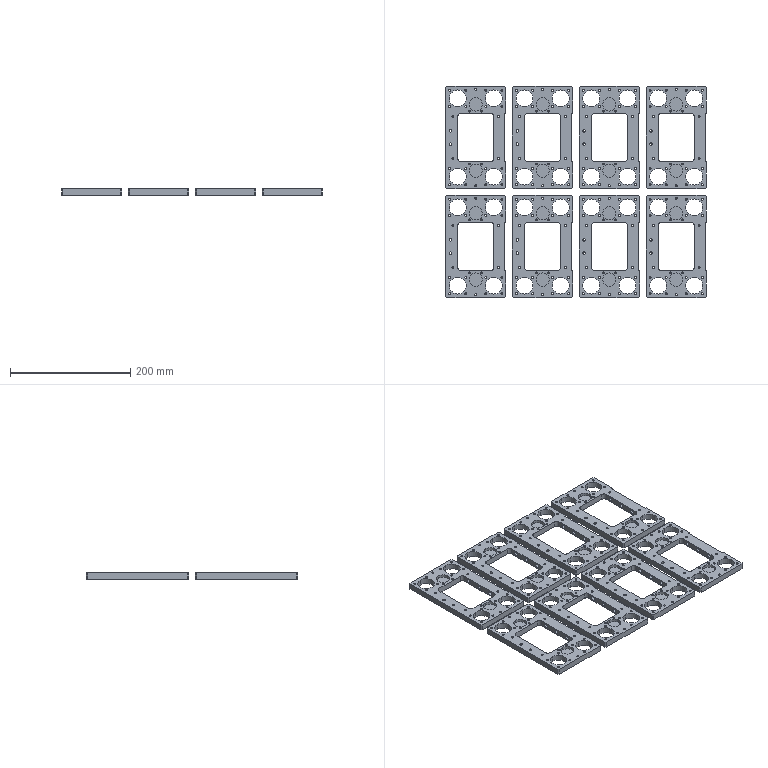Part | 8 solids | 784 faces | box 433 x 351 x 10 mm | volume 701074 mm3 | cylinder 624 | plane 160 | commonest cylinder face diameters 3.3 x416 28.1 x64 6.5 x48 4.2 x32 10 x32 22 x32